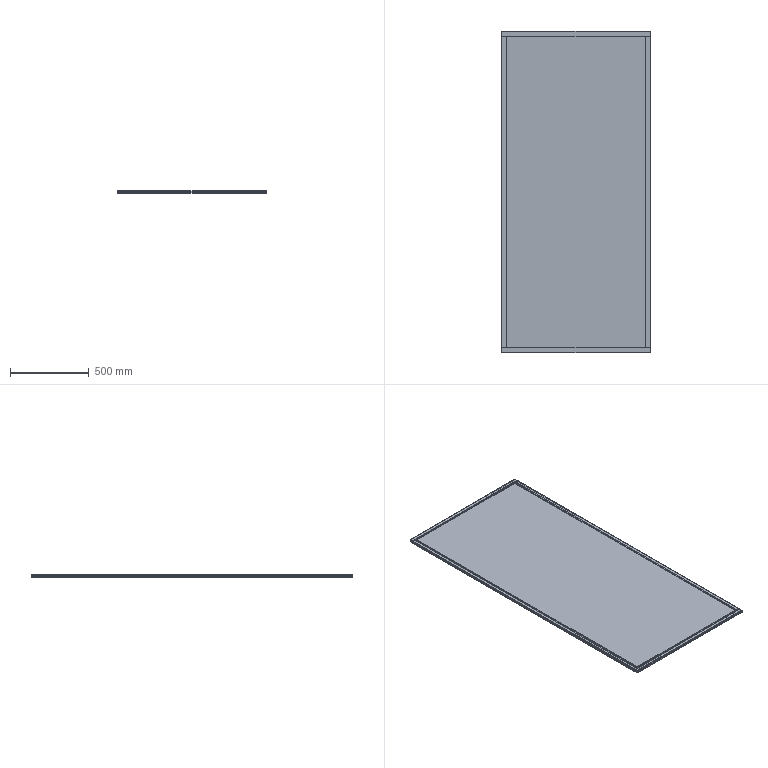Part | 5 solids | 167 faces | box 940 x 2036 x 18 mm | volume 19006527 mm3 | plane 98 | cylinder 69 | commonest cylinder face diameters 1.1 x24 3.6 x20 5.8 x20 1 x5